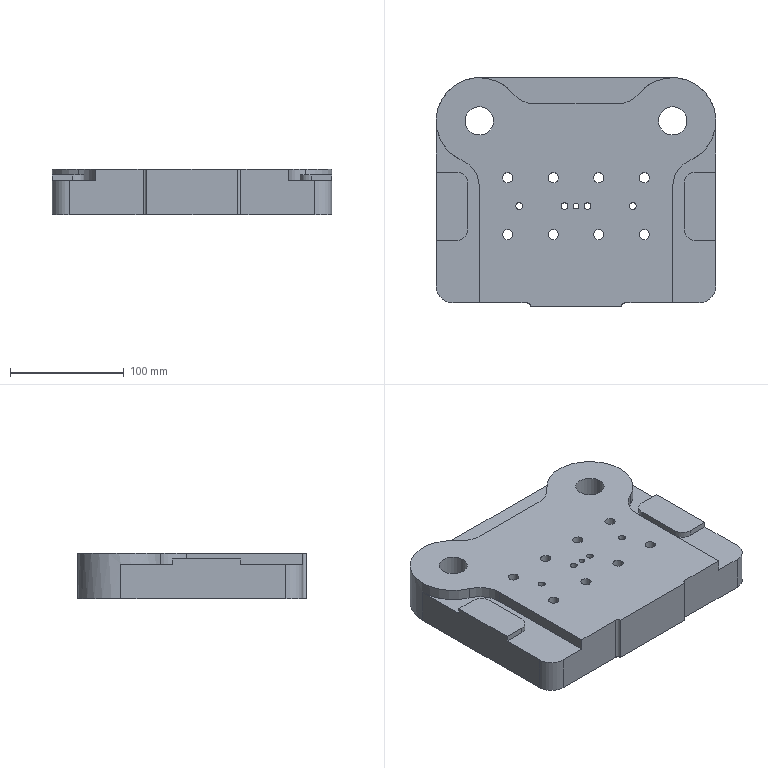Part | NX | features EXTRUDE 5, DATUM_CSYS 1 | 1 solid | 67 faces | box 246 x 201 x 40 mm | volume 1748151 mm3 | cylinder 37 | plane 30 | commonest cylinder face diameters 9 x8 15 x8 6 x6 20 x4 50 x4 25 x2